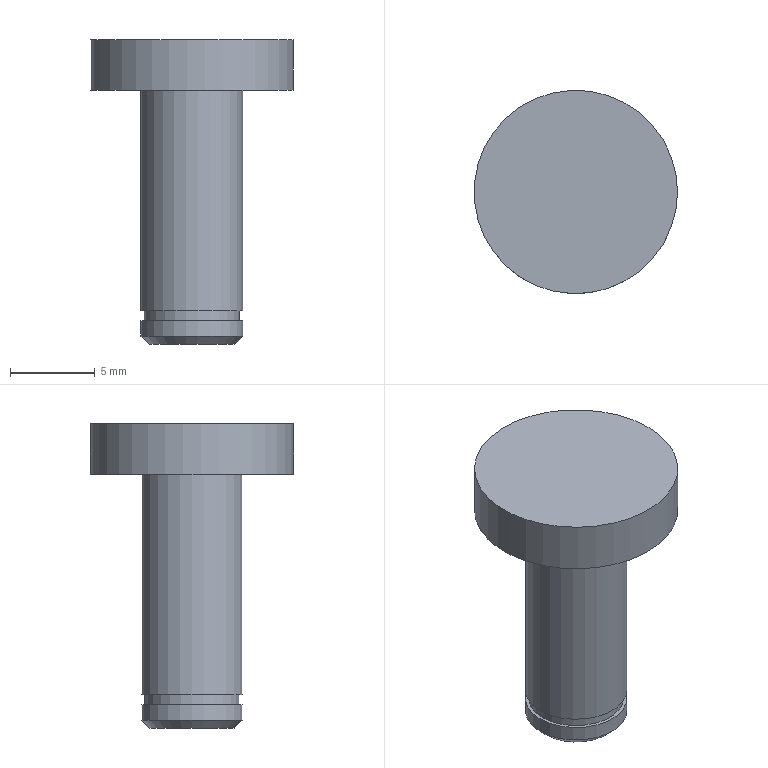Part | NX | features BREP 1, DATUM_CSYS 1 | 1 solid | 10 faces | box 12 x 12 x 18 mm | volume 758.995 mm3 | plane 5 | cylinder 4 | cone 1 | commonest cylinder face diameters 6 x2 5.6 x1 12 x1
STEP:
#1=CARTESIAN_POINT('',(6.,0.,18.));
#2=VERTEX_POINT('',#1);
#3=CARTESIAN_POINT('',(0.,0.,18.));
#4=DIRECTION('',(0.,0.,1.));
#5=DIRECTION('',(1.,0.,0.));
#6=AXIS2_PLACEMENT_3D('',#3,#4,#5);
#7=CIRCLE('',#6,6.);
#8=EDGE_CURVE('',#2,#2,#7,.T.);
#9=ORIENTED_EDGE('',*,*,#8,.T.);
#10=EDGE_LOOP('',(#9));
#11=FACE_BOUND('',#10,.T.);
#12=CARTESIAN_POINT('',(0.,0.,18.));
#13=DIRECTION('',(0.,0.,1.));
#14=DIRECTION('',(-1.,0.,0.));
#15=AXIS2_PLACEMENT_3D('',#12,#13,#14);
#16=PLANE('',#15);
#17=ADVANCED_FACE('',(#11),#16,.T.);
#18=CARTESIAN_POINT('',(6.,0.,15.));
#19=VERTEX_POINT('',#18);
#20=CARTESIAN_POINT('',(0.,0.,15.));
#21=DIRECTION('',(0.,0.,1.));
#22=DIRECTION('',(1.,0.,0.));
#23=AXIS2_PLACEMENT_3D('',#20,#21,#22);
#24=CIRCLE('',#23,6.);
#25=EDGE_CURVE('',#19,#19,#24,.T.);
#26=ORIENTED_EDGE('',*,*,#25,.T.);
#27=CARTESIAN_POINT('',(6.,0.,15.));
#28=DIRECTION('',(0.,0.,1.));
#29=VECTOR('',#28,1000.);
#30=LINE('',#27,#29);
#31=EDGE_CURVE('',#19,#2,#30,.T.);
#32=ORIENTED_EDGE('',*,*,#31,.T.);
#33=ORIENTED_EDGE('',*,*,#8,.F.);
#34=ORIENTED_EDGE('',*,*,#31,.F.);
#35=EDGE_LOOP('',(#26,#32,#33,#34));
#36=FACE_BOUND('',#35,.T.);
#37=CARTESIAN_POINT('',(0.,0.,15.));
#38=DIRECTION('',(0.,0.,1.));
#39=DIRECTION('',(-1.,0.,0.));
#40=AXIS2_PLACEMENT_3D('',#37,#38,#39);
#41=CYLINDRICAL_SURFACE('',#40,6.);
#42=ADVANCED_FACE('',(#36),#41,.T.);
#43=ORIENTED_EDGE('',*,*,#25,.F.);
#44=EDGE_LOOP('',(#43));
#45=FACE_BOUND('',#44,.T.);
#46=CARTESIAN_POINT('',(3.,0.,15.));
#47=VERTEX_POINT('',#46);
#48=CARTESIAN_POINT('',(0.,0.,15.));
#49=DIRECTION('',(0.,0.,1.));
#50=DIRECTION('',(1.,0.,0.));
#51=AXIS2_PLACEMENT_3D('',#48,#49,#50);
#52=CIRCLE('',#51,3.);
#53=EDGE_CURVE('',#47,#47,#52,.T.);
#54=ORIENTED_EDGE('',*,*,#53,.T.);
#55=EDGE_LOOP('',(#54));
#56=FACE_BOUND('',#55,.T.);
#57=CARTESIAN_POINT('',(0.,0.,15.));
#58=DIRECTION('',(0.,0.,1.));
#59=DIRECTION('',(-1.,0.,0.));
#60=AXIS2_PLACEMENT_3D('',#57,#58,#59);
#61=PLANE('',#60);
#62=ADVANCED_FACE('',(#45,#56),#61,.F.);
#63=CARTESIAN_POINT('',(2.5,0.,0.));
#64=VERTEX_POINT('',#63);
#65=CARTESIAN_POINT('',(0.,0.,0.));
#66=DIRECTION('',(0.,0.,-1.));
#67=DIRECTION('',(1.,0.,0.));
#68=AXIS2_PLACEMENT_3D('',#65,#66,#67);
#69=CIRCLE('',#68,2.5);
#70=EDGE_CURVE('',#64,#64,#69,.T.);
#71=ORIENTED_EDGE('',*,*,#70,.T.);
#72=EDGE_LOOP('',(#71));
#73=FACE_BOUND('',#72,.T.);
#74=CARTESIAN_POINT('',(0.,0.,0.));
#75=DIRECTION('',(0.,0.,1.));
#76=DIRECTION('',(-1.,0.,0.));
#77=AXIS2_PLACEMENT_3D('',#74,#75,#76);
#78=PLANE('',#77);
#79=ADVANCED_FACE('',(#73),#78,.F.);
#80=CARTESIAN_POINT('',(3.,0.,1.4));
#81=VERTEX_POINT('',#80);
#82=CARTESIAN_POINT('',(0.,0.,1.4));
#83=DIRECTION('',(0.,0.,1.));
#84=DIRECTION('',(1.,0.,0.));
#85=AXIS2_PLACEMENT_3D('',#82,#83,#84);
#86=CIRCLE('',#85,3.);
#87=EDGE_CURVE('',#81,#81,#86,.T.);
#88=ORIENTED_EDGE('',*,*,#87,.F.);
#89=CARTESIAN_POINT('',(3.,0.,0.5));
#90=VERTEX_POINT('',#89);
#91=CARTESIAN_POINT('',(3.,0.,0.5));
#92=DIRECTION('',(0.,0.,1.));
#93=VECTOR('',#92,1000.);
#94=LINE('',#91,#93);
#95=EDGE_CURVE('',#90,#81,#94,.T.);
#96=ORIENTED_EDGE('',*,*,#95,.F.);
#97=CARTESIAN_POINT('',(0.,0.,0.5));
#98=DIRECTION('',(0.,0.,-1.));
#99=DIRECTION('',(1.,0.,0.));
#100=AXIS2_PLACEMENT_3D('',#97,#98,#99);
#101=CIRCLE('',#100,3.);
#102=EDGE_CURVE('',#90,#90,#101,.T.);
#103=ORIENTED_EDGE('',*,*,#102,.F.);
#104=ORIENTED_EDGE('',*,*,#95,.T.);
#105=EDGE_LOOP('',(#88,#96,#103,#104));
#106=FACE_BOUND('',#105,.T.);
#107=CARTESIAN_POINT('',(0.,0.,0.));
#108=DIRECTION('',(0.,0.,1.));
#109=DIRECTION('',(-1.,0.,0.));
#110=AXIS2_PLACEMENT_3D('',#107,#108,#109);
#111=CYLINDRICAL_SURFACE('',#110,3.);
#112=ADVANCED_FACE('',(#106),#111,.T.);
#113=ORIENTED_EDGE('',*,*,#53,.F.);
#114=CARTESIAN_POINT('',(3.,0.,2.));
#115=VERTEX_POINT('',#114);
#116=CARTESIAN_POINT('',(3.,0.,2.));
#117=DIRECTION('',(0.,0.,1.));
#118=VECTOR('',#117,1000.);
#119=LINE('',#116,#118);
#120=EDGE_CURVE('',#115,#47,#119,.T.);
#121=ORIENTED_EDGE('',*,*,#120,.F.);
#122=CARTESIAN_POINT('',(0.,0.,2.));
#123=DIRECTION('',(0.,0.,-1.));
#124=DIRECTION('',(1.,0.,0.));
#125=AXIS2_PLACEMENT_3D('',#122,#123,#124);
#126=CIRCLE('',#125,3.);
#127=EDGE_CURVE('',#115,#115,#126,.T.);
#128=ORIENTED_EDGE('',*,*,#127,.F.);
#129=ORIENTED_EDGE('',*,*,#120,.T.);
#130=EDGE_LOOP('',(#113,#121,#128,#129));
#131=FACE_BOUND('',#130,.T.);
#132=CARTESIAN_POINT('',(0.,0.,0.));
#133=DIRECTION('',(0.,0.,1.));
#134=DIRECTION('',(-1.,0.,0.));
#135=AXIS2_PLACEMENT_3D('',#132,#133,#134);
#136=CYLINDRICAL_SURFACE('',#135,3.);
#137=ADVANCED_FACE('',(#131),#136,.T.);
#138=ORIENTED_EDGE('',*,*,#127,.T.);
#139=EDGE_LOOP('',(#138));
#140=FACE_BOUND('',#139,.T.);
#141=CARTESIAN_POINT('',(2.8,0.,2.));
#142=VERTEX_POINT('',#141);
#143=CARTESIAN_POINT('',(0.,0.,2.));
#144=DIRECTION('',(0.,0.,-1.));
#145=DIRECTION('',(1.,0.,0.));
#146=AXIS2_PLACEMENT_3D('',#143,#144,#145);
#147=CIRCLE('',#146,2.8);
#148=EDGE_CURVE('',#142,#142,#147,.T.);
#149=ORIENTED_EDGE('',*,*,#148,.F.);
#150=EDGE_LOOP('',(#149));
#151=FACE_BOUND('',#150,.T.);
#152=CARTESIAN_POINT('',(0.,0.,2.));
#153=DIRECTION('',(0.,0.,1.));
#154=DIRECTION('',(-1.,0.,0.));
#155=AXIS2_PLACEMENT_3D('',#152,#153,#154);
#156=PLANE('',#155);
#157=ADVANCED_FACE('',(#140,#151),#156,.F.);
#158=ORIENTED_EDGE('',*,*,#148,.T.);
#159=CARTESIAN_POINT('',(2.8,0.,1.4));
#160=VERTEX_POINT('',#159);
#161=CARTESIAN_POINT('',(2.8,0.,2.));
#162=DIRECTION('',(0.,0.,-1.));
#163=VECTOR('',#162,1000.);
#164=LINE('',#161,#163);
#165=EDGE_CURVE('',#142,#160,#164,.T.);
#166=ORIENTED_EDGE('',*,*,#165,.T.);
#167=CARTESIAN_POINT('',(0.,0.,1.4));
#168=DIRECTION('',(0.,0.,-1.));
#169=DIRECTION('',(1.,0.,0.));
#170=AXIS2_PLACEMENT_3D('',#167,#168,#169);
#171=CIRCLE('',#170,2.8);
#172=EDGE_CURVE('',#160,#160,#171,.T.);
#173=ORIENTED_EDGE('',*,*,#172,.F.);
#174=ORIENTED_EDGE('',*,*,#165,.F.);
#175=EDGE_LOOP('',(#158,#166,#173,#174));
#176=FACE_BOUND('',#175,.T.);
#177=CARTESIAN_POINT('',(0.,0.,2.));
#178=DIRECTION('',(0.,0.,-1.));
#179=DIRECTION('',(-1.,0.,0.));
#180=AXIS2_PLACEMENT_3D('',#177,#178,#179);
#181=CYLINDRICAL_SURFACE('',#180,2.8);
#182=ADVANCED_FACE('',(#176),#181,.T.);
#183=ORIENTED_EDGE('',*,*,#87,.T.);
#184=EDGE_LOOP('',(#183));
#185=FACE_BOUND('',#184,.T.);
#186=ORIENTED_EDGE('',*,*,#172,.T.);
#187=EDGE_LOOP('',(#186));
#188=FACE_BOUND('',#187,.T.);
#189=CARTESIAN_POINT('',(0.,0.,1.4));
#190=DIRECTION('',(0.,0.,-1.));
#191=DIRECTION('',(-1.,0.,0.));
#192=AXIS2_PLACEMENT_3D('',#189,#190,#191);
#193=PLANE('',#192);
#194=ADVANCED_FACE('',(#185,#188),#193,.F.);
#195=ORIENTED_EDGE('',*,*,#70,.F.);
#196=CARTESIAN_POINT('',(2.5,0.,0.));
#197=DIRECTION('',(0.7071,0.,0.7071));
#198=VECTOR('',#197,1000.);
#199=LINE('',#196,#198);
#200=EDGE_CURVE('',#64,#90,#199,.T.);
#201=ORIENTED_EDGE('',*,*,#200,.T.);
#202=ORIENTED_EDGE('',*,*,#102,.T.);
#203=ORIENTED_EDGE('',*,*,#200,.F.);
#204=EDGE_LOOP('',(#195,#201,#202,#203));
#205=FACE_BOUND('',#204,.T.);
#206=CARTESIAN_POINT('',(0.,0.,0.));
#207=DIRECTION('',(0.,0.,1.));
#208=DIRECTION('',(-1.,0.,0.));
#209=AXIS2_PLACEMENT_3D('',#206,#207,#208);
#210=CONICAL_SURFACE('',#209,2.5,0.7854);
#211=ADVANCED_FACE('',(#205),#210,.T.);
#212=CLOSED_SHELL('',(#17,#42,#62,#79,#112,#137,#157,#182,#194,#211));
#213=MANIFOLD_SOLID_BREP('',#212);
#214=(LENGTH_UNIT()NAMED_UNIT(*)SI_UNIT(.MILLI.,.METRE.));
#215=UNCERTAINTY_MEASURE_WITH_UNIT(LENGTH_MEASURE(0.00001),#214,'','');
#216=(NAMED_UNIT(*)PLANE_ANGLE_UNIT()SI_UNIT($,.RADIAN.));
#217=(NAMED_UNIT(*)SI_UNIT($,.STERADIAN.)SOLID_ANGLE_UNIT());
#218=(GEOMETRIC_REPRESENTATION_CONTEXT(3)GLOBAL_UNCERTAINTY_ASSIGNED_CONTEXT((#215))GLOBAL_UNIT_ASSIGNED_CONTEXT((#214,#216,#217))REPRESENTATION_CONTEXT('',''));
#219=ADVANCED_BREP_SHAPE_REPRESENTATION('',(#213),#218);